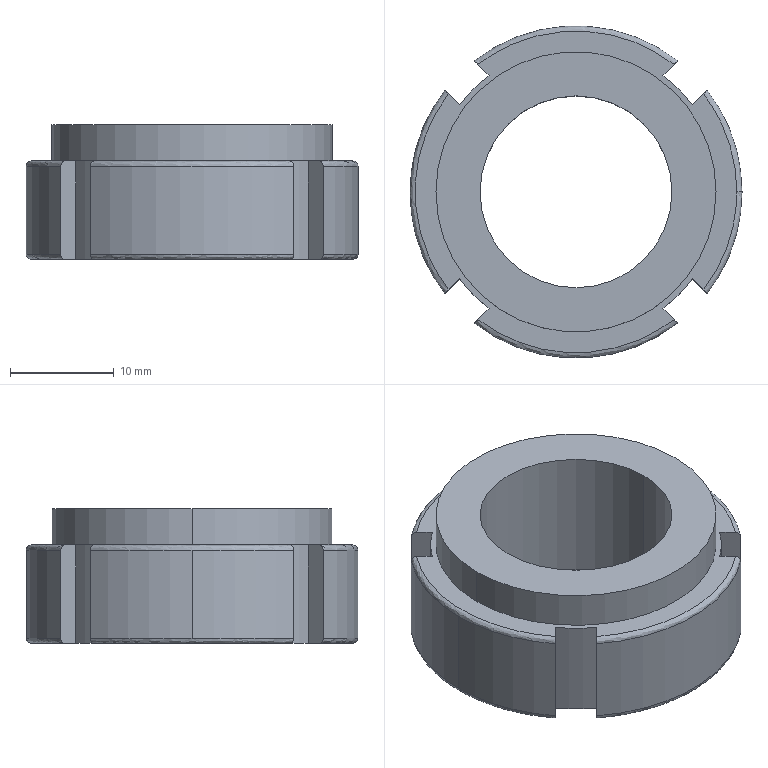Part | SolidWorks | features BaseBody 1, MoveFace 1 | 1 solid | 34 faces | box 32 x 32 x 13 mm | volume 5836 mm3 | cylinder 13 | plane 11 | spline 10 | commonest cylinder face diameters 32 x5 28 x4 18.5 x2 27 x2